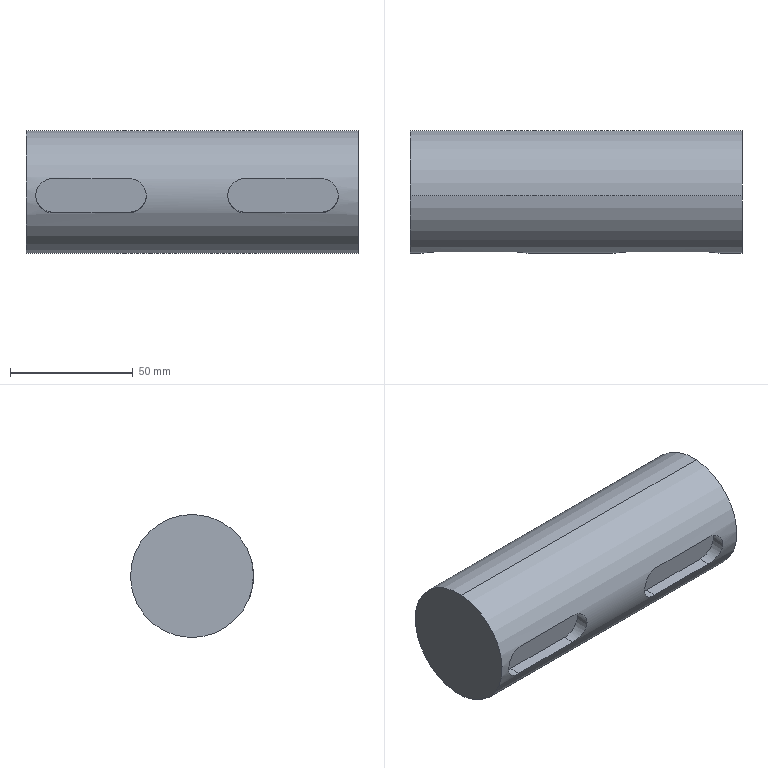Part | STEP file | Cut-Extrude 1-1 | 1 solid | 14 faces | box 135 x 50 x 50 mm | volume 258968 mm3 | plane 8 | cylinder 6 | commonest cylinder face diameters 14 x4 50 x2
STEP:
#1=CARTESIAN_POINT('',(-102.476,-512.81,2433.285));
#2=VERTEX_POINT('',#1);
#3=CARTESIAN_POINT('',(-102.476,-513.697,2447.257));
#4=VERTEX_POINT('',#3);
#5=CARTESIAN_POINT('',(-102.476,-512.81,2433.285));
#6=CARTESIAN_POINT('',(-102.011,-512.81,2433.285));
#7=CARTESIAN_POINT('',(-101.555,-512.826,2433.33));
#8=CARTESIAN_POINT('',(-100.882,-512.873,2433.462));
#9=CARTESIAN_POINT('',(-100.659,-512.892,2433.516));
#10=CARTESIAN_POINT('',(-100.218,-512.938,2433.648));
#11=CARTESIAN_POINT('',(-100.,-512.965,2433.725));
#12=CARTESIAN_POINT('',(-99.365,-513.052,2433.984));
#13=CARTESIAN_POINT('',(-98.964,-513.121,2434.195));
#14=CARTESIAN_POINT('',(-98.395,-513.236,2434.569));
#15=CARTESIAN_POINT('',(-98.21,-513.276,2434.704));
#16=CARTESIAN_POINT('',(-97.856,-513.359,2434.99));
#17=CARTESIAN_POINT('',(-97.687,-513.401,2435.141));
#18=CARTESIAN_POINT('',(-97.206,-513.529,2435.615));
#19=CARTESIAN_POINT('',(-96.917,-513.615,2435.961));
#20=CARTESIAN_POINT('',(-96.405,-513.784,2436.716));
#21=CARTESIAN_POINT('',(-96.189,-513.864,2437.116));
#22=CARTESIAN_POINT('',(-95.926,-513.972,2437.741));
#23=CARTESIAN_POINT('',(-95.849,-514.006,2437.954));
#24=CARTESIAN_POINT('',(-95.715,-514.07,2438.39));
#25=CARTESIAN_POINT('',(-95.658,-514.1,2438.614));
#26=CARTESIAN_POINT('',(-95.522,-514.18,2439.289));
#27=CARTESIAN_POINT('',(-95.477,-514.222,2439.743));
#28=CARTESIAN_POINT('',(-95.476,-514.28,2440.659));
#29=CARTESIAN_POINT('',(-95.522,-514.297,2441.126));
#30=CARTESIAN_POINT('',(-95.701,-514.305,2442.026));
#31=CARTESIAN_POINT('',(-95.834,-514.296,2442.465));
#32=CARTESIAN_POINT('',(-96.098,-514.268,2443.106));
#33=CARTESIAN_POINT('',(-96.197,-514.256,2443.317));
#34=CARTESIAN_POINT('',(-96.413,-514.228,2443.723));
#35=CARTESIAN_POINT('',(-96.531,-514.212,2443.919));
#36=CARTESIAN_POINT('',(-96.783,-514.176,2444.3));
#37=CARTESIAN_POINT('',(-96.919,-514.157,2444.484));
#38=CARTESIAN_POINT('',(-97.208,-514.116,2444.841));
#39=CARTESIAN_POINT('',(-97.363,-514.094,2445.014));
#40=CARTESIAN_POINT('',(-97.848,-514.027,2445.504));
#41=CARTESIAN_POINT('',(-98.199,-513.981,2445.796));
#42=CARTESIAN_POINT('',(-98.954,-513.892,2446.309));
#43=CARTESIAN_POINT('',(-99.364,-513.849,2446.533));
#44=CARTESIAN_POINT('',(-100.208,-513.777,2446.889));
#45=CARTESIAN_POINT('',(-100.644,-513.748,2447.025));
#46=CARTESIAN_POINT('',(-101.321,-513.718,2447.163));
#47=CARTESIAN_POINT('',(-101.551,-513.71,2447.199));
#48=CARTESIAN_POINT('',(-102.012,-513.7,2447.245));
#49=CARTESIAN_POINT('',(-102.244,-513.697,2447.257));
#50=CARTESIAN_POINT('',(-102.476,-513.697,2447.257));
#51=B_SPLINE_CURVE_WITH_KNOTS('',3,(#5,#6,#7,#8,#9,#10,#11,#12,#13,#14,#15,#16,#17,#18,#19,#20,#21,#22,#23,#24,#25,#26,#27,#28,#29,#30,#31,#32,#33,#34,#35,#36,#37,#38,#39,#40,#41,#42,#43,#44,#45,#46,#47,#48,#49,#50),.UNSPECIFIED.,.F.,.F.,(4,2,2,2,2,2,2,2,2,2,2,2,2,2,2,2,2,2,2,2,2,2,4),(0.,0.001374,0.002061,0.002749,0.004123,0.00481,0.005497,0.006871,0.008246,0.008933,0.00962,0.01099,0.01237,0.01374,0.01443,0.01512,0.0158,0.01649,0.01787,0.01924,0.02061,0.0213,0.02199),.UNSPECIFIED.);
#52=EDGE_CURVE('',#2,#4,#51,.T.);
#53=ORIENTED_EDGE('',*,*,#52,.F.);
#54=CARTESIAN_POINT('',(-133.476,-512.81,2433.285));
#55=VERTEX_POINT('',#54);
#56=CARTESIAN_POINT('',(-9.407,-512.81,2433.285));
#57=DIRECTION('',(1.,0.,0.));
#58=VECTOR('',#57,1000.);
#59=LINE('',#56,#58);
#60=EDGE_CURVE('',#55,#2,#59,.T.);
#61=ORIENTED_EDGE('',*,*,#60,.F.);
#62=CARTESIAN_POINT('',(-133.476,-513.697,2447.257));
#63=VERTEX_POINT('',#62);
#64=CARTESIAN_POINT('',(-133.476,-513.697,2447.257));
#65=CARTESIAN_POINT('',(-133.941,-513.697,2447.257));
#66=CARTESIAN_POINT('',(-134.398,-513.708,2447.21));
#67=CARTESIAN_POINT('',(-135.071,-513.738,2447.074));
#68=CARTESIAN_POINT('',(-135.293,-513.75,2447.017));
#69=CARTESIAN_POINT('',(-135.734,-513.779,2446.881));
#70=CARTESIAN_POINT('',(-135.953,-513.795,2446.801));
#71=CARTESIAN_POINT('',(-136.587,-513.849,2446.533));
#72=CARTESIAN_POINT('',(-136.988,-513.891,2446.315));
#73=CARTESIAN_POINT('',(-137.558,-513.957,2445.929));
#74=CARTESIAN_POINT('',(-137.743,-513.98,2445.79));
#75=CARTESIAN_POINT('',(-138.097,-514.026,2445.496));
#76=CARTESIAN_POINT('',(-138.265,-514.049,2445.341));
#77=CARTESIAN_POINT('',(-138.747,-514.116,2444.855));
#78=CARTESIAN_POINT('',(-139.036,-514.158,2444.5));
#79=CARTESIAN_POINT('',(-139.548,-514.23,2443.73));
#80=CARTESIAN_POINT('',(-139.764,-514.258,2443.324));
#81=CARTESIAN_POINT('',(-140.026,-514.287,2442.69));
#82=CARTESIAN_POINT('',(-140.104,-514.293,2442.474));
#83=CARTESIAN_POINT('',(-140.238,-514.302,2442.034));
#84=CARTESIAN_POINT('',(-140.295,-514.303,2441.807));
#85=CARTESIAN_POINT('',(-140.431,-514.297,2441.128));
#86=CARTESIAN_POINT('',(-140.476,-514.281,2440.672));
#87=CARTESIAN_POINT('',(-140.477,-514.223,2439.756));
#88=CARTESIAN_POINT('',(-140.431,-514.18,2439.292));
#89=CARTESIAN_POINT('',(-140.251,-514.074,2438.397));
#90=CARTESIAN_POINT('',(-140.119,-514.01,2437.962));
#91=CARTESIAN_POINT('',(-139.854,-513.901,2437.33));
#92=CARTESIAN_POINT('',(-139.755,-513.863,2437.123));
#93=CARTESIAN_POINT('',(-139.539,-513.784,2436.724));
#94=CARTESIAN_POINT('',(-139.422,-513.743,2436.531));
#95=CARTESIAN_POINT('',(-139.169,-513.659,2436.158));
#96=CARTESIAN_POINT('',(-139.034,-513.617,2435.977));
#97=CARTESIAN_POINT('',(-138.744,-513.531,2435.629));
#98=CARTESIAN_POINT('',(-138.589,-513.487,2435.46));
#99=CARTESIAN_POINT('',(-138.104,-513.359,2434.982));
#100=CARTESIAN_POINT('',(-137.754,-513.276,2434.699));
#101=CARTESIAN_POINT('',(-136.998,-513.123,2434.201));
#102=CARTESIAN_POINT('',(-136.588,-513.052,2433.984));
#103=CARTESIAN_POINT('',(-135.745,-512.936,2433.64));
#104=CARTESIAN_POINT('',(-135.309,-512.89,2433.509));
#105=CARTESIAN_POINT('',(-134.632,-512.842,2433.375));
#106=CARTESIAN_POINT('',(-134.402,-512.83,2433.342));
#107=CARTESIAN_POINT('',(-133.94,-512.814,2433.296));
#108=CARTESIAN_POINT('',(-133.709,-512.81,2433.285));
#109=CARTESIAN_POINT('',(-133.476,-512.81,2433.285));
#110=B_SPLINE_CURVE_WITH_KNOTS('',3,(#64,#65,#66,#67,#68,#69,#70,#71,#72,#73,#74,#75,#76,#77,#78,#79,#80,#81,#82,#83,#84,#85,#86,#87,#88,#89,#90,#91,#92,#93,#94,#95,#96,#97,#98,#99,#100,#101,#102,#103,#104,#105,#106,#107,#108,#109),.UNSPECIFIED.,.F.,.F.,(4,2,2,2,2,2,2,2,2,2,2,2,2,2,2,2,2,2,2,2,2,2,4),(0.,0.001374,0.002061,0.002749,0.004123,0.00481,0.005497,0.006871,0.008246,0.008933,0.00962,0.01099,0.01237,0.01374,0.01443,0.01512,0.0158,0.01649,0.01787,0.01924,0.02061,0.0213,0.02199),.UNSPECIFIED.);
#111=EDGE_CURVE('',#63,#55,#110,.T.);
#112=ORIENTED_EDGE('',*,*,#111,.F.);
#113=CARTESIAN_POINT('',(-9.407,-513.697,2447.257));
#114=DIRECTION('',(-1.,0.,0.));
#115=VECTOR('',#114,1000.);
#116=LINE('',#113,#115);
#117=EDGE_CURVE('',#4,#63,#116,.T.);
#118=ORIENTED_EDGE('',*,*,#117,.F.);
#119=EDGE_LOOP('',(#53,#61,#112,#118));
#120=FACE_BOUND('',#119,.T.);
#121=CARTESIAN_POINT('',(-24.407,-512.81,2433.285));
#122=VERTEX_POINT('',#121);
#123=CARTESIAN_POINT('',(-24.407,-513.697,2447.257));
#124=VERTEX_POINT('',#123);
#125=CARTESIAN_POINT('',(-24.407,-512.81,2433.285));
#126=CARTESIAN_POINT('',(-23.942,-512.81,2433.285));
#127=CARTESIAN_POINT('',(-23.485,-512.826,2433.33));
#128=CARTESIAN_POINT('',(-22.812,-512.873,2433.462));
#129=CARTESIAN_POINT('',(-22.589,-512.892,2433.516));
#130=CARTESIAN_POINT('',(-22.149,-512.938,2433.648));
#131=CARTESIAN_POINT('',(-21.93,-512.965,2433.725));
#132=CARTESIAN_POINT('',(-21.295,-513.052,2433.984));
#133=CARTESIAN_POINT('',(-20.894,-513.121,2434.195));
#134=CARTESIAN_POINT('',(-20.325,-513.236,2434.569));
#135=CARTESIAN_POINT('',(-20.14,-513.276,2434.704));
#136=CARTESIAN_POINT('',(-19.786,-513.359,2434.99));
#137=CARTESIAN_POINT('',(-19.617,-513.401,2435.141));
#138=CARTESIAN_POINT('',(-19.136,-513.529,2435.615));
#139=CARTESIAN_POINT('',(-18.847,-513.615,2435.961));
#140=CARTESIAN_POINT('',(-18.335,-513.784,2436.716));
#141=CARTESIAN_POINT('',(-18.119,-513.864,2437.116));
#142=CARTESIAN_POINT('',(-17.856,-513.972,2437.741));
#143=CARTESIAN_POINT('',(-17.779,-514.006,2437.954));
#144=CARTESIAN_POINT('',(-17.645,-514.07,2438.39));
#145=CARTESIAN_POINT('',(-17.588,-514.1,2438.614));
#146=CARTESIAN_POINT('',(-17.452,-514.18,2439.289));
#147=CARTESIAN_POINT('',(-17.407,-514.222,2439.743));
#148=CARTESIAN_POINT('',(-17.406,-514.28,2440.659));
#149=CARTESIAN_POINT('',(-17.452,-514.297,2441.126));
#150=CARTESIAN_POINT('',(-17.631,-514.305,2442.026));
#151=CARTESIAN_POINT('',(-17.764,-514.296,2442.465));
#152=CARTESIAN_POINT('',(-18.029,-514.268,2443.106));
#153=CARTESIAN_POINT('',(-18.128,-514.256,2443.317));
#154=CARTESIAN_POINT('',(-18.344,-514.228,2443.723));
#155=CARTESIAN_POINT('',(-18.461,-514.212,2443.919));
#156=CARTESIAN_POINT('',(-18.714,-514.176,2444.3));
#157=CARTESIAN_POINT('',(-18.849,-514.157,2444.484));
#158=CARTESIAN_POINT('',(-19.138,-514.116,2444.841));
#159=CARTESIAN_POINT('',(-19.293,-514.094,2445.014));
#160=CARTESIAN_POINT('',(-19.778,-514.027,2445.504));
#161=CARTESIAN_POINT('',(-20.129,-513.981,2445.796));
#162=CARTESIAN_POINT('',(-20.885,-513.892,2446.309));
#163=CARTESIAN_POINT('',(-21.294,-513.849,2446.533));
#164=CARTESIAN_POINT('',(-22.138,-513.777,2446.889));
#165=CARTESIAN_POINT('',(-22.574,-513.748,2447.025));
#166=CARTESIAN_POINT('',(-23.251,-513.718,2447.163));
#167=CARTESIAN_POINT('',(-23.481,-513.71,2447.199));
#168=CARTESIAN_POINT('',(-23.943,-513.7,2447.245));
#169=CARTESIAN_POINT('',(-24.174,-513.697,2447.257));
#170=CARTESIAN_POINT('',(-24.407,-513.697,2447.257));
#171=B_SPLINE_CURVE_WITH_KNOTS('',3,(#125,#126,#127,#128,#129,#130,#131,#132,#133,#134,#135,#136,#137,#138,#139,#140,#141,#142,#143,#144,#145,#146,#147,#148,#149,#150,#151,#152,#153,#154,#155,#156,#157,#158,#159,#160,#161,#162,#163,#164,#165,#166,#167,#168,#169,#170),.UNSPECIFIED.,.F.,.F.,(4,2,2,2,2,2,2,2,2,2,2,2,2,2,2,2,2,2,2,2,2,2,4),(0.,0.001374,0.002061,0.002749,0.004123,0.00481,0.005497,0.006871,0.008246,0.008933,0.00962,0.01099,0.01237,0.01374,0.01443,0.01512,0.0158,0.01649,0.01787,0.01924,0.02061,0.0213,0.02199),.UNSPECIFIED.);
#172=EDGE_CURVE('',#122,#124,#171,.T.);
#173=ORIENTED_EDGE('',*,*,#172,.F.);
#174=CARTESIAN_POINT('',(-55.407,-512.81,2433.285));
#175=VERTEX_POINT('',#174);
#176=CARTESIAN_POINT('',(-9.407,-512.81,2433.285));
#177=DIRECTION('',(1.,0.,0.));
#178=VECTOR('',#177,1000.);
#179=LINE('',#176,#178);
#180=EDGE_CURVE('',#175,#122,#179,.T.);
#181=ORIENTED_EDGE('',*,*,#180,.F.);
#182=CARTESIAN_POINT('',(-55.407,-513.697,2447.257));
#183=VERTEX_POINT('',#182);
#184=CARTESIAN_POINT('',(-55.407,-513.697,2447.257));
#185=CARTESIAN_POINT('',(-55.871,-513.697,2447.257));
#186=CARTESIAN_POINT('',(-56.328,-513.708,2447.21));
#187=CARTESIAN_POINT('',(-57.001,-513.738,2447.074));
#188=CARTESIAN_POINT('',(-57.224,-513.75,2447.017));
#189=CARTESIAN_POINT('',(-57.664,-513.779,2446.881));
#190=CARTESIAN_POINT('',(-57.883,-513.795,2446.801));
#191=CARTESIAN_POINT('',(-58.518,-513.849,2446.533));
#192=CARTESIAN_POINT('',(-58.919,-513.891,2446.315));
#193=CARTESIAN_POINT('',(-59.488,-513.957,2445.929));
#194=CARTESIAN_POINT('',(-59.673,-513.98,2445.79));
#195=CARTESIAN_POINT('',(-60.027,-514.026,2445.496));
#196=CARTESIAN_POINT('',(-60.196,-514.049,2445.341));
#197=CARTESIAN_POINT('',(-60.677,-514.116,2444.855));
#198=CARTESIAN_POINT('',(-60.966,-514.158,2444.5));
#199=CARTESIAN_POINT('',(-61.478,-514.23,2443.73));
#200=CARTESIAN_POINT('',(-61.694,-514.258,2443.324));
#201=CARTESIAN_POINT('',(-61.957,-514.287,2442.69));
#202=CARTESIAN_POINT('',(-62.034,-514.293,2442.474));
#203=CARTESIAN_POINT('',(-62.168,-514.302,2442.034));
#204=CARTESIAN_POINT('',(-62.225,-514.303,2441.807));
#205=CARTESIAN_POINT('',(-62.361,-514.297,2441.128));
#206=CARTESIAN_POINT('',(-62.406,-514.281,2440.672));
#207=CARTESIAN_POINT('',(-62.407,-514.223,2439.756));
#208=CARTESIAN_POINT('',(-62.361,-514.18,2439.292));
#209=CARTESIAN_POINT('',(-62.182,-514.074,2438.397));
#210=CARTESIAN_POINT('',(-62.049,-514.01,2437.962));
#211=CARTESIAN_POINT('',(-61.784,-513.901,2437.33));
#212=CARTESIAN_POINT('',(-61.685,-513.863,2437.123));
#213=CARTESIAN_POINT('',(-61.469,-513.784,2436.724));
#214=CARTESIAN_POINT('',(-61.352,-513.743,2436.531));
#215=CARTESIAN_POINT('',(-61.099,-513.659,2436.158));
#216=CARTESIAN_POINT('',(-60.964,-513.617,2435.977));
#217=CARTESIAN_POINT('',(-60.675,-513.531,2435.629));
#218=CARTESIAN_POINT('',(-60.52,-513.487,2435.46));
#219=CARTESIAN_POINT('',(-60.035,-513.359,2434.982));
#220=CARTESIAN_POINT('',(-59.684,-513.276,2434.699));
#221=CARTESIAN_POINT('',(-58.928,-513.123,2434.201));
#222=CARTESIAN_POINT('',(-58.519,-513.052,2433.984));
#223=CARTESIAN_POINT('',(-57.675,-512.936,2433.64));
#224=CARTESIAN_POINT('',(-57.239,-512.89,2433.509));
#225=CARTESIAN_POINT('',(-56.562,-512.842,2433.375));
#226=CARTESIAN_POINT('',(-56.332,-512.83,2433.342));
#227=CARTESIAN_POINT('',(-55.871,-512.814,2433.296));
#228=CARTESIAN_POINT('',(-55.639,-512.81,2433.285));
#229=CARTESIAN_POINT('',(-55.407,-512.81,2433.285));
#230=B_SPLINE_CURVE_WITH_KNOTS('',3,(#184,#185,#186,#187,#188,#189,#190,#191,#192,#193,#194,#195,#196,#197,#198,#199,#200,#201,#202,#203,#204,#205,#206,#207,#208,#209,#210,#211,#212,#213,#214,#215,#216,#217,#218,#219,#220,#221,#222,#223,#224,#225,#226,#227,#228,#229),.UNSPECIFIED.,.F.,.F.,(4,2,2,2,2,2,2,2,2,2,2,2,2,2,2,2,2,2,2,2,2,2,4),(0.,0.001374,0.002061,0.002749,0.004123,0.00481,0.005497,0.006871,0.008246,0.008933,0.00962,0.01099,0.01237,0.01374,0.01443,0.01512,0.0158,0.01649,0.01787,0.01924,0.02061,0.0213,0.02199),.UNSPECIFIED.);
#231=EDGE_CURVE('',#183,#175,#230,.T.);
#232=ORIENTED_EDGE('',*,*,#231,.F.);
#233=CARTESIAN_POINT('',(-9.407,-513.697,2447.257));
#234=DIRECTION('',(-1.,0.,0.));
#235=VECTOR('',#234,1000.);
#236=LINE('',#233,#235);
#237=EDGE_CURVE('',#124,#183,#236,.T.);
#238=ORIENTED_EDGE('',*,*,#237,.F.);
#239=EDGE_LOOP('',(#173,#181,#232,#238));
#240=FACE_BOUND('',#239,.T.);
#241=CARTESIAN_POINT('',(-144.407,-490.886,2466.742));
#242=VERTEX_POINT('',#241);
#243=CARTESIAN_POINT('',(-144.407,-487.717,2416.843));
#244=VERTEX_POINT('',#243);
#245=CARTESIAN_POINT('',(-144.407,-489.302,2441.792));
#246=DIRECTION('',(1.,0.,0.));
#247=DIRECTION('',(0.,-0.06338,0.998));
#248=AXIS2_PLACEMENT_3D('',#245,#246,#247);
#249=CIRCLE('',#248,25.);
#250=EDGE_CURVE('',#242,#244,#249,.T.);
#251=ORIENTED_EDGE('',*,*,#250,.T.);
#252=CARTESIAN_POINT('',(-9.407,-487.717,2416.843));
#253=VERTEX_POINT('',#252);
#254=CARTESIAN_POINT('',(-9.407,-487.717,2416.843));
#255=DIRECTION('',(1.,0.,0.));
#256=VECTOR('',#255,1000.);
#257=LINE('',#254,#256);
#258=EDGE_CURVE('',#244,#253,#257,.T.);
#259=ORIENTED_EDGE('',*,*,#258,.T.);
#260=CARTESIAN_POINT('',(-9.407,-490.886,2466.742));
#261=VERTEX_POINT('',#260);
#262=CARTESIAN_POINT('',(-9.407,-489.302,2441.792));
#263=DIRECTION('',(1.,0.,0.));
#264=DIRECTION('',(0.,-0.06338,0.998));
#265=AXIS2_PLACEMENT_3D('',#262,#263,#264);
#266=CIRCLE('',#265,25.);
#267=EDGE_CURVE('',#261,#253,#266,.T.);
#268=ORIENTED_EDGE('',*,*,#267,.F.);
#269=CARTESIAN_POINT('',(-9.407,-490.886,2466.742));
#270=DIRECTION('',(1.,0.,0.));
#271=VECTOR('',#270,1000.);
#272=LINE('',#269,#271);
#273=EDGE_CURVE('',#242,#261,#272,.T.);
#274=ORIENTED_EDGE('',*,*,#273,.F.);
#275=EDGE_LOOP('',(#251,#259,#268,#274));
#276=FACE_OUTER_BOUND('',#275,.T.);
#277=CARTESIAN_POINT('',(-9.407,-489.302,2441.792));
#278=DIRECTION('',(1.,0.,0.));
#279=DIRECTION('',(0.,0.06338,-0.998));
#280=AXIS2_PLACEMENT_3D('',#277,#278,#279);
#281=CYLINDRICAL_SURFACE('',#280,25.);
#282=ADVANCED_FACE('',(#120,#240,#276),#281,.T.);
#283=ORIENTED_EDGE('',*,*,#258,.F.);
#284=CARTESIAN_POINT('',(-144.407,-489.302,2441.792));
#285=DIRECTION('',(1.,0.,0.));
#286=DIRECTION('',(0.,-0.06338,0.998));
#287=AXIS2_PLACEMENT_3D('',#284,#285,#286);
#288=CIRCLE('',#287,25.);
#289=EDGE_CURVE('',#244,#242,#288,.T.);
#290=ORIENTED_EDGE('',*,*,#289,.T.);
#291=ORIENTED_EDGE('',*,*,#273,.T.);
#292=CARTESIAN_POINT('',(-9.407,-489.302,2441.792));
#293=DIRECTION('',(1.,0.,0.));
#294=DIRECTION('',(0.,-0.06338,0.998));
#295=AXIS2_PLACEMENT_3D('',#292,#293,#294);
#296=CIRCLE('',#295,25.);
#297=EDGE_CURVE('',#253,#261,#296,.T.);
#298=ORIENTED_EDGE('',*,*,#297,.F.);
#299=EDGE_LOOP('',(#283,#290,#291,#298));
#300=FACE_OUTER_BOUND('',#299,.T.);
#301=CARTESIAN_POINT('',(-9.407,-489.302,2441.792));
#302=DIRECTION('',(1.,0.,0.));
#303=DIRECTION('',(0.,0.06338,-0.998));
#304=AXIS2_PLACEMENT_3D('',#301,#302,#303);
#305=CYLINDRICAL_SURFACE('',#304,25.);
#306=ADVANCED_FACE('',(#300),#305,.T.);
#307=ORIENTED_EDGE('',*,*,#267,.T.);
#308=ORIENTED_EDGE('',*,*,#297,.T.);
#309=EDGE_LOOP('',(#307,#308));
#310=FACE_OUTER_BOUND('',#309,.T.);
#311=CARTESIAN_POINT('',(-9.407,-489.302,2441.792));
#312=DIRECTION('',(-1.,0.,0.));
#313=DIRECTION('',(0.,-0.06338,0.998));
#314=AXIS2_PLACEMENT_3D('',#311,#312,#313);
#315=PLANE('',#314);
#316=ADVANCED_FACE('',(#310),#315,.F.);
#317=ORIENTED_EDGE('',*,*,#250,.F.);
#318=ORIENTED_EDGE('',*,*,#289,.F.);
#319=EDGE_LOOP('',(#317,#318));
#320=FACE_OUTER_BOUND('',#319,.T.);
#321=CARTESIAN_POINT('',(-144.407,-514.252,2440.208));
#322=DIRECTION('',(1.,0.,0.));
#323=DIRECTION('',(0.,0.06338,-0.998));
#324=AXIS2_PLACEMENT_3D('',#321,#322,#323);
#325=PLANE('',#324);
#326=ADVANCED_FACE('',(#320),#325,.F.);
#327=ORIENTED_EDGE('',*,*,#52,.T.);
#328=CARTESIAN_POINT('',(-102.476,-509.206,2447.542));
#329=VERTEX_POINT('',#328);
#330=CARTESIAN_POINT('',(-102.476,-519.186,2446.908));
#331=DIRECTION('',(0.,0.998,0.06338));
#332=VECTOR('',#331,1000.);
#333=LINE('',#330,#332);
#334=EDGE_CURVE('',#4,#329,#333,.T.);
#335=ORIENTED_EDGE('',*,*,#334,.T.);
#336=CARTESIAN_POINT('',(-102.476,-508.319,2433.57));
#337=VERTEX_POINT('',#336);
#338=CARTESIAN_POINT('',(-102.476,-508.763,2440.556));
#339=DIRECTION('',(0.,-0.998,-0.06338));
#340=DIRECTION('',(0.,-0.06338,0.998));
#341=AXIS2_PLACEMENT_3D('',#338,#339,#340);
#342=CIRCLE('',#341,7.);
#343=EDGE_CURVE('',#337,#329,#342,.T.);
#344=ORIENTED_EDGE('',*,*,#343,.F.);
#345=CARTESIAN_POINT('',(-102.476,-518.299,2432.937));
#346=DIRECTION('',(0.,0.998,0.06338));
#347=VECTOR('',#346,1000.);
#348=LINE('',#345,#347);
#349=EDGE_CURVE('',#2,#337,#348,.T.);
#350=ORIENTED_EDGE('',*,*,#349,.F.);
#351=EDGE_LOOP('',(#327,#335,#344,#350));
#352=FACE_OUTER_BOUND('',#351,.T.);
#353=CARTESIAN_POINT('',(-102.476,-518.742,2439.922));
#354=DIRECTION('',(0.,0.998,0.06338));
#355=DIRECTION('',(0.,-0.06338,0.998));
#356=AXIS2_PLACEMENT_3D('',#353,#354,#355);
#357=CYLINDRICAL_SURFACE('',#356,7.);
#358=ADVANCED_FACE('',(#352),#357,.F.);
#359=ORIENTED_EDGE('',*,*,#117,.T.);
#360=CARTESIAN_POINT('',(-133.476,-509.206,2447.542));
#361=VERTEX_POINT('',#360);
#362=CARTESIAN_POINT('',(-133.476,-519.186,2446.908));
#363=DIRECTION('',(0.,0.998,0.06338));
#364=VECTOR('',#363,1000.);
#365=LINE('',#362,#364);
#366=EDGE_CURVE('',#63,#361,#365,.T.);
#367=ORIENTED_EDGE('',*,*,#366,.T.);
#368=CARTESIAN_POINT('',(-102.476,-509.206,2447.542));
#369=DIRECTION('',(-1.,0.,0.));
#370=VECTOR('',#369,1000.);
#371=LINE('',#368,#370);
#372=EDGE_CURVE('',#329,#361,#371,.T.);
#373=ORIENTED_EDGE('',*,*,#372,.F.);
#374=ORIENTED_EDGE('',*,*,#334,.F.);
#375=EDGE_LOOP('',(#359,#367,#373,#374));
#376=FACE_OUTER_BOUND('',#375,.T.);
#377=CARTESIAN_POINT('',(-102.476,-519.186,2446.908));
#378=DIRECTION('',(0.,0.06338,-0.998));
#379=DIRECTION('',(-1.,0.,0.));
#380=AXIS2_PLACEMENT_3D('',#377,#378,#379);
#381=PLANE('',#380);
#382=ADVANCED_FACE('',(#376),#381,.T.);
#383=ORIENTED_EDGE('',*,*,#111,.T.);
#384=CARTESIAN_POINT('',(-133.476,-508.319,2433.57));
#385=VERTEX_POINT('',#384);
#386=CARTESIAN_POINT('',(-133.476,-518.299,2432.937));
#387=DIRECTION('',(0.,0.998,0.06338));
#388=VECTOR('',#387,1000.);
#389=LINE('',#386,#388);
#390=EDGE_CURVE('',#55,#385,#389,.T.);
#391=ORIENTED_EDGE('',*,*,#390,.T.);
#392=CARTESIAN_POINT('',(-133.476,-508.763,2440.556));
#393=DIRECTION('',(0.,-0.998,-0.06338));
#394=DIRECTION('',(0.,-0.06338,0.998));
#395=AXIS2_PLACEMENT_3D('',#392,#393,#394);
#396=CIRCLE('',#395,7.);
#397=EDGE_CURVE('',#361,#385,#396,.T.);
#398=ORIENTED_EDGE('',*,*,#397,.F.);
#399=ORIENTED_EDGE('',*,*,#366,.F.);
#400=EDGE_LOOP('',(#383,#391,#398,#399));
#401=FACE_OUTER_BOUND('',#400,.T.);
#402=CARTESIAN_POINT('',(-133.476,-518.742,2439.922));
#403=DIRECTION('',(0.,0.998,0.06338));
#404=DIRECTION('',(0.,-0.06338,0.998));
#405=AXIS2_PLACEMENT_3D('',#402,#403,#404);
#406=CYLINDRICAL_SURFACE('',#405,7.);
#407=ADVANCED_FACE('',(#401),#406,.F.);
#408=ORIENTED_EDGE('',*,*,#60,.T.);
#409=ORIENTED_EDGE('',*,*,#349,.T.);
#410=CARTESIAN_POINT('',(-102.476,-508.319,2433.57));
#411=DIRECTION('',(1.,0.,0.));
#412=VECTOR('',#411,1000.);
#413=LINE('',#410,#412);
#414=EDGE_CURVE('',#385,#337,#413,.T.);
#415=ORIENTED_EDGE('',*,*,#414,.F.);
#416=ORIENTED_EDGE('',*,*,#390,.F.);
#417=EDGE_LOOP('',(#408,#409,#415,#416));
#418=FACE_OUTER_BOUND('',#417,.T.);
#419=CARTESIAN_POINT('',(-102.476,-518.299,2432.937));
#420=DIRECTION('',(0.,-0.06338,0.998));
#421=DIRECTION('',(1.,0.,0.));
#422=AXIS2_PLACEMENT_3D('',#419,#420,#421);
#423=PLANE('',#422);
#424=ADVANCED_FACE('',(#418),#423,.T.);
#425=ORIENTED_EDGE('',*,*,#343,.T.);
#426=ORIENTED_EDGE('',*,*,#372,.T.);
#427=ORIENTED_EDGE('',*,*,#397,.T.);
#428=ORIENTED_EDGE('',*,*,#414,.T.);
#429=EDGE_LOOP('',(#425,#426,#427,#428));
#430=FACE_OUTER_BOUND('',#429,.T.);
#431=CARTESIAN_POINT('',(-102.476,-508.763,2440.556));
#432=DIRECTION('',(0.,-0.998,-0.06338));
#433=DIRECTION('',(0.,0.06338,-0.998));
#434=AXIS2_PLACEMENT_3D('',#431,#432,#433);
#435=PLANE('',#434);
#436=ADVANCED_FACE('',(#430),#435,.T.);
#437=ORIENTED_EDGE('',*,*,#172,.T.);
#438=CARTESIAN_POINT('',(-24.407,-509.206,2447.542));
#439=VERTEX_POINT('',#438);
#440=CARTESIAN_POINT('',(-24.407,-519.186,2446.908));
#441=DIRECTION('',(0.,0.998,0.06338));
#442=VECTOR('',#441,1000.);
#443=LINE('',#440,#442);
#444=EDGE_CURVE('',#124,#439,#443,.T.);
#445=ORIENTED_EDGE('',*,*,#444,.T.);
#446=CARTESIAN_POINT('',(-24.407,-508.319,2433.57));
#447=VERTEX_POINT('',#446);
#448=CARTESIAN_POINT('',(-24.407,-508.763,2440.556));
#449=DIRECTION('',(0.,-0.998,-0.06338));
#450=DIRECTION('',(0.,-0.06338,0.998));
#451=AXIS2_PLACEMENT_3D('',#448,#449,#450);
#452=CIRCLE('',#451,7.);
#453=EDGE_CURVE('',#447,#439,#452,.T.);
#454=ORIENTED_EDGE('',*,*,#453,.F.);
#455=CARTESIAN_POINT('',(-24.407,-518.299,2432.937));
#456=DIRECTION('',(0.,0.998,0.06338));
#457=VECTOR('',#456,1000.);
#458=LINE('',#455,#457);
#459=EDGE_CURVE('',#122,#447,#458,.T.);
#460=ORIENTED_EDGE('',*,*,#459,.F.);
#461=EDGE_LOOP('',(#437,#445,#454,#460));
#462=FACE_OUTER_BOUND('',#461,.T.);
#463=CARTESIAN_POINT('',(-24.407,-518.742,2439.922));
#464=DIRECTION('',(0.,0.998,0.06338));
#465=DIRECTION('',(0.,-0.06338,0.998));
#466=AXIS2_PLACEMENT_3D('',#463,#464,#465);
#467=CYLINDRICAL_SURFACE('',#466,7.);
#468=ADVANCED_FACE('',(#462),#467,.F.);
#469=ORIENTED_EDGE('',*,*,#237,.T.);
#470=CARTESIAN_POINT('',(-55.407,-509.206,2447.542));
#471=VERTEX_POINT('',#470);
#472=CARTESIAN_POINT('',(-55.407,-519.186,2446.908));
#473=DIRECTION('',(0.,0.998,0.06338));
#474=VECTOR('',#473,1000.);
#475=LINE('',#472,#474);
#476=EDGE_CURVE('',#183,#471,#475,.T.);
#477=ORIENTED_EDGE('',*,*,#476,.T.);
#478=CARTESIAN_POINT('',(-24.407,-509.206,2447.542));
#479=DIRECTION('',(-1.,0.,0.));
#480=VECTOR('',#479,1000.);
#481=LINE('',#478,#480);
#482=EDGE_CURVE('',#439,#471,#481,.T.);
#483=ORIENTED_EDGE('',*,*,#482,.F.);
#484=ORIENTED_EDGE('',*,*,#444,.F.);
#485=EDGE_LOOP('',(#469,#477,#483,#484));
#486=FACE_OUTER_BOUND('',#485,.T.);
#487=CARTESIAN_POINT('',(-24.407,-519.186,2446.908));
#488=DIRECTION('',(0.,0.06338,-0.998));
#489=DIRECTION('',(-1.,0.,0.));
#490=AXIS2_PLACEMENT_3D('',#487,#488,#489);
#491=PLANE('',#490);
#492=ADVANCED_FACE('',(#486),#491,.T.);
#493=ORIENTED_EDGE('',*,*,#231,.T.);
#494=CARTESIAN_POINT('',(-55.407,-508.319,2433.57));
#495=VERTEX_POINT('',#494);
#496=CARTESIAN_POINT('',(-55.407,-518.299,2432.937));
#497=DIRECTION('',(0.,0.998,0.06338));
#498=VECTOR('',#497,1000.);
#499=LINE('',#496,#498);
#500=EDGE_CURVE('',#175,#495,#499,.T.);
#501=ORIENTED_EDGE('',*,*,#500,.T.);
#502=CARTESIAN_POINT('',(-55.407,-508.763,2440.556));
#503=DIRECTION('',(0.,-0.998,-0.06338));
#504=DIRECTION('',(0.,-0.06338,0.998));
#505=AXIS2_PLACEMENT_3D('',#502,#503,#504);
#506=CIRCLE('',#505,7.);
#507=EDGE_CURVE('',#471,#495,#506,.T.);
#508=ORIENTED_EDGE('',*,*,#507,.F.);
#509=ORIENTED_EDGE('',*,*,#476,.F.);
#510=EDGE_LOOP('',(#493,#501,#508,#509));
#511=FACE_OUTER_BOUND('',#510,.T.);
#512=CARTESIAN_POINT('',(-55.407,-518.742,2439.922));
#513=DIRECTION('',(0.,0.998,0.06338));
#514=DIRECTION('',(0.,-0.06338,0.998));
#515=AXIS2_PLACEMENT_3D('',#512,#513,#514);
#516=CYLINDRICAL_SURFACE('',#515,7.);
#517=ADVANCED_FACE('',(#511),#516,.F.);
#518=ORIENTED_EDGE('',*,*,#180,.T.);
#519=ORIENTED_EDGE('',*,*,#459,.T.);
#520=CARTESIAN_POINT('',(-24.407,-508.319,2433.57));
#521=DIRECTION('',(1.,0.,0.));
#522=VECTOR('',#521,1000.);
#523=LINE('',#520,#522);
#524=EDGE_CURVE('',#495,#447,#523,.T.);
#525=ORIENTED_EDGE('',*,*,#524,.F.);
#526=ORIENTED_EDGE('',*,*,#500,.F.);
#527=EDGE_LOOP('',(#518,#519,#525,#526));
#528=FACE_OUTER_BOUND('',#527,.T.);
#529=CARTESIAN_POINT('',(-24.407,-518.299,2432.937));
#530=DIRECTION('',(0.,-0.06338,0.998));
#531=DIRECTION('',(1.,0.,0.));
#532=AXIS2_PLACEMENT_3D('',#529,#530,#531);
#533=PLANE('',#532);
#534=ADVANCED_FACE('',(#528),#533,.T.);
#535=ORIENTED_EDGE('',*,*,#453,.T.);
#536=ORIENTED_EDGE('',*,*,#482,.T.);
#537=ORIENTED_EDGE('',*,*,#507,.T.);
#538=ORIENTED_EDGE('',*,*,#524,.T.);
#539=EDGE_LOOP('',(#535,#536,#537,#538));
#540=FACE_OUTER_BOUND('',#539,.T.);
#541=CARTESIAN_POINT('',(-24.407,-508.763,2440.556));
#542=DIRECTION('',(0.,-0.998,-0.06338));
#543=DIRECTION('',(0.,0.06338,-0.998));
#544=AXIS2_PLACEMENT_3D('',#541,#542,#543);
#545=PLANE('',#544);
#546=ADVANCED_FACE('',(#540),#545,.T.);
#547=CLOSED_SHELL('',(#282,#306,#316,#326,#358,#382,#407,#424,#436,#468,#492,#517,#534,#546));
#548=MANIFOLD_SOLID_BREP('',#547);
#549=CARTESIAN_POINT('',(0.,0.,0.));
#550=DIRECTION('',(0.,0.,1.));
#551=DIRECTION('',(1.,0.,0.));
#552=AXIS2_PLACEMENT_3D('',#549,#550,#551);
#553=(LENGTH_UNIT()NAMED_UNIT(*)SI_UNIT(.MILLI.,.METRE.));
#554=UNCERTAINTY_MEASURE_WITH_UNIT(LENGTH_MEASURE(0.00001),#553,'','');
#555=(NAMED_UNIT(*)PLANE_ANGLE_UNIT()SI_UNIT($,.RADIAN.));
#556=(NAMED_UNIT(*)SI_UNIT($,.STERADIAN.)SOLID_ANGLE_UNIT());
#557=(GEOMETRIC_REPRESENTATION_CONTEXT(3)GLOBAL_UNCERTAINTY_ASSIGNED_CONTEXT((#554))GLOBAL_UNIT_ASSIGNED_CONTEXT((#553,#555,#556))REPRESENTATION_CONTEXT('',''));
#558=ADVANCED_BREP_SHAPE_REPRESENTATION('',(#548,#552),#557);